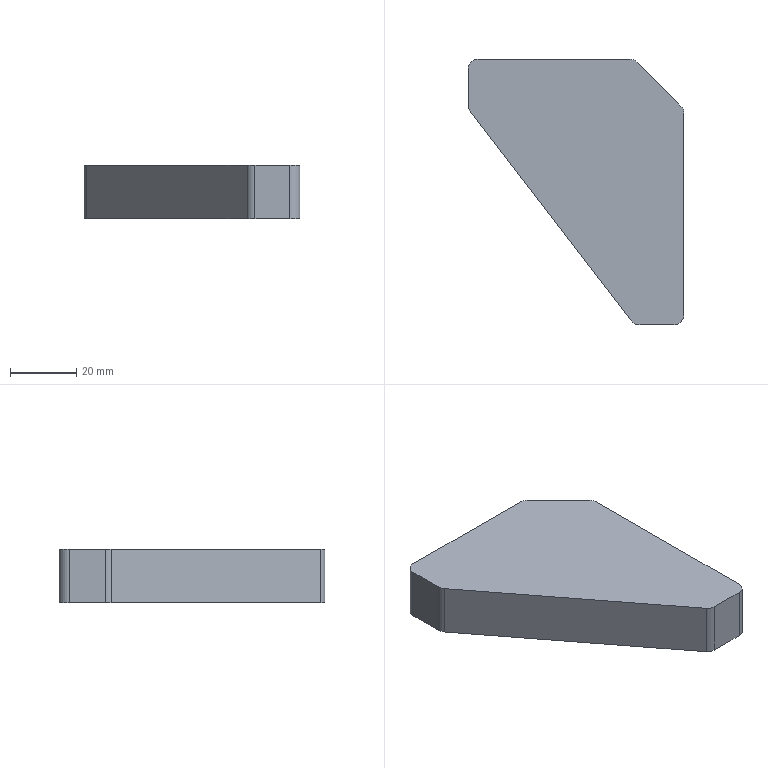Part | STEP file | SN10_008_007-03_REFORCO | 1 solid | 14 faces | box 65 x 80 x 16 mm | volume 55325 mm3 | plane 8 | cylinder 6 | commonest cylinder face diameters 6 x6
STEP:
#1=CARTESIAN_POINT('',(0.,0.,0.));
#2=DIRECTION('',(0.,0.,1.));
#3=DIRECTION('',(1.,0.,0.));
#4=AXIS2_PLACEMENT_3D('',#1,#2,#3);
#5=CARTESIAN_POINT('',(243.629,237.,420.27));
#6=VERTEX_POINT('',#5);
#7=CARTESIAN_POINT('',(246.629,240.,420.27));
#8=VERTEX_POINT('',#7);
#9=CARTESIAN_POINT('',(246.629,237.,420.27));
#10=DIRECTION('',(0.,0.,-1.));
#11=DIRECTION('',(1.,0.,0.));
#12=AXIS2_PLACEMENT_3D('',#9,#10,#11);
#13=CIRCLE('',#12,3.);
#14=CARTESIAN_POINT('',(246.629,237.,428.27));
#15=DIRECTION('',(0.,0.,-1.));
#16=DIRECTION('',(-1.,0.,0.));
#17=AXIS2_PLACEMENT_3D('',#14,#15,#16);
#18=CYLINDRICAL_SURFACE('',#17,3.);
#19=CARTESIAN_POINT('',(-3.142,8.));
#20=DIRECTION('',(1.,0.));
#21=VECTOR('',#20,1.);
#22=LINE('',#19,#21);
#23=(GEOMETRIC_REPRESENTATION_CONTEXT(2)PARAMETRIC_REPRESENTATION_CONTEXT()REPRESENTATION_CONTEXT('',''));
#24=DEFINITIONAL_REPRESENTATION('',(#22),#23);
#25=PCURVE('',#18,#24);
#26=CARTESIAN_POINT('',(0.,0.,420.27));
#27=DIRECTION('',(0.,0.,-1.));
#28=DIRECTION('',(-1.,0.,0.));
#29=AXIS2_PLACEMENT_3D('',#26,#27,#28);
#30=PLANE('',#29);
#31=CARTESIAN_POINT('',(-246.629,237.));
#32=DIRECTION('',(-1.,0.));
#33=AXIS2_PLACEMENT_2D('',#31,#32);
#34=CIRCLE('',#33,3.);
#35=(GEOMETRIC_REPRESENTATION_CONTEXT(2)PARAMETRIC_REPRESENTATION_CONTEXT()REPRESENTATION_CONTEXT('',''));
#36=DEFINITIONAL_REPRESENTATION('',(#34),#35);
#37=PCURVE('',#30,#36);
#38=SURFACE_CURVE('',#13,(#25,#37),.PCURVE_S1.);
#39=EDGE_CURVE('',#6,#8,#38,.T.);
#40=ORIENTED_EDGE('',*,*,#39,.F.);
#41=CARTESIAN_POINT('',(243.629,237.,436.27));
#42=VERTEX_POINT('',#41);
#43=CARTESIAN_POINT('',(243.629,237.,436.27));
#44=DIRECTION('',(0.,0.,-1.));
#45=VECTOR('',#44,1.);
#46=LINE('',#43,#45);
#47=CARTESIAN_POINT('',(0.,-8.));
#48=DIRECTION('',(0.,1.));
#49=VECTOR('',#48,1.);
#50=LINE('',#47,#49);
#51=(GEOMETRIC_REPRESENTATION_CONTEXT(2)PARAMETRIC_REPRESENTATION_CONTEXT()REPRESENTATION_CONTEXT('',''));
#52=DEFINITIONAL_REPRESENTATION('',(#50),#51);
#53=PCURVE('',#18,#52);
#54=CARTESIAN_POINT('',(243.629,225.,436.27));
#55=DIRECTION('',(-1.,0.,0.));
#56=DIRECTION('',(0.,0.,1.));
#57=AXIS2_PLACEMENT_3D('',#54,#55,#56);
#58=PLANE('',#57);
#59=CARTESIAN_POINT('',(0.,12.));
#60=DIRECTION('',(-1.,0.));
#61=VECTOR('',#60,1.);
#62=LINE('',#59,#61);
#63=(GEOMETRIC_REPRESENTATION_CONTEXT(2)PARAMETRIC_REPRESENTATION_CONTEXT()REPRESENTATION_CONTEXT('',''));
#64=DEFINITIONAL_REPRESENTATION('',(#62),#63);
#65=PCURVE('',#58,#64);
#66=SURFACE_CURVE('',#46,(#53,#65),.PCURVE_S1.);
#67=EDGE_CURVE('',#42,#6,#66,.T.);
#68=ORIENTED_EDGE('',*,*,#67,.F.);
#69=CARTESIAN_POINT('',(246.629,240.,436.27));
#70=VERTEX_POINT('',#69);
#71=CARTESIAN_POINT('',(246.629,237.,436.27));
#72=DIRECTION('',(0.,0.,-1.));
#73=DIRECTION('',(1.,0.,0.));
#74=AXIS2_PLACEMENT_3D('',#71,#72,#73);
#75=CIRCLE('',#74,3.);
#76=CARTESIAN_POINT('',(-3.142,-8.));
#77=DIRECTION('',(1.,0.));
#78=VECTOR('',#77,1.);
#79=LINE('',#76,#78);
#80=(GEOMETRIC_REPRESENTATION_CONTEXT(2)PARAMETRIC_REPRESENTATION_CONTEXT()REPRESENTATION_CONTEXT('',''));
#81=DEFINITIONAL_REPRESENTATION('',(#79),#80);
#82=PCURVE('',#18,#81);
#83=CARTESIAN_POINT('',(0.,0.,436.27));
#84=DIRECTION('',(0.,0.,-1.));
#85=DIRECTION('',(-1.,0.,0.));
#86=AXIS2_PLACEMENT_3D('',#83,#84,#85);
#87=PLANE('',#86);
#88=CARTESIAN_POINT('',(-246.629,237.));
#89=DIRECTION('',(-1.,0.));
#90=AXIS2_PLACEMENT_2D('',#88,#89);
#91=CIRCLE('',#90,3.);
#92=(GEOMETRIC_REPRESENTATION_CONTEXT(2)PARAMETRIC_REPRESENTATION_CONTEXT()REPRESENTATION_CONTEXT('',''));
#93=DEFINITIONAL_REPRESENTATION('',(#91),#92);
#94=PCURVE('',#87,#93);
#95=SURFACE_CURVE('',#75,(#82,#94),.PCURVE_S1.);
#96=EDGE_CURVE('',#42,#70,#95,.T.);
#97=ORIENTED_EDGE('',*,*,#96,.T.);
#98=CARTESIAN_POINT('',(246.629,240.,436.27));
#99=DIRECTION('',(0.,0.,-1.));
#100=VECTOR('',#99,1.);
#101=LINE('',#98,#100);
#102=CARTESIAN_POINT('',(1.571,-8.));
#103=DIRECTION('',(0.,1.));
#104=VECTOR('',#103,1.);
#105=LINE('',#102,#104);
#106=(GEOMETRIC_REPRESENTATION_CONTEXT(2)PARAMETRIC_REPRESENTATION_CONTEXT()REPRESENTATION_CONTEXT('',''));
#107=DEFINITIONAL_REPRESENTATION('',(#105),#106);
#108=PCURVE('',#18,#107);
#109=CARTESIAN_POINT('',(243.629,240.,436.27));
#110=DIRECTION('',(0.,1.,0.));
#111=DIRECTION('',(0.,0.,1.));
#112=AXIS2_PLACEMENT_3D('',#109,#110,#111);
#113=PLANE('',#112);
#114=CARTESIAN_POINT('',(0.,3.));
#115=DIRECTION('',(-1.,0.));
#116=VECTOR('',#115,1.);
#117=LINE('',#114,#116);
#118=(GEOMETRIC_REPRESENTATION_CONTEXT(2)PARAMETRIC_REPRESENTATION_CONTEXT()REPRESENTATION_CONTEXT('',''));
#119=DEFINITIONAL_REPRESENTATION('',(#117),#118);
#120=PCURVE('',#113,#119);
#121=SURFACE_CURVE('',#101,(#108,#120),.PCURVE_S1.);
#122=EDGE_CURVE('',#70,#8,#121,.T.);
#123=ORIENTED_EDGE('',*,*,#122,.T.);
#124=EDGE_LOOP('',(#40,#68,#97,#123));
#125=FACE_BOUND('',#124,.T.);
#126=ADVANCED_FACE('',(#125),#18,.T.);
#127=CARTESIAN_POINT('',(243.629,226.02,436.27));
#128=VERTEX_POINT('',#127);
#129=CARTESIAN_POINT('',(243.629,226.02,436.27));
#130=DIRECTION('',(0.,1.,0.));
#131=VECTOR('',#130,1.);
#132=LINE('',#129,#131);
#133=CARTESIAN_POINT('',(0.,1.02));
#134=DIRECTION('',(0.,1.));
#135=VECTOR('',#134,1.);
#136=LINE('',#133,#135);
#137=(GEOMETRIC_REPRESENTATION_CONTEXT(2)PARAMETRIC_REPRESENTATION_CONTEXT()REPRESENTATION_CONTEXT('',''));
#138=DEFINITIONAL_REPRESENTATION('',(#136),#137);
#139=PCURVE('',#58,#138);
#140=CARTESIAN_POINT('',(-243.629,226.02));
#141=DIRECTION('',(0.,1.));
#142=VECTOR('',#141,1.);
#143=LINE('',#140,#142);
#144=(GEOMETRIC_REPRESENTATION_CONTEXT(2)PARAMETRIC_REPRESENTATION_CONTEXT()REPRESENTATION_CONTEXT('',''));
#145=DEFINITIONAL_REPRESENTATION('',(#143),#144);
#146=PCURVE('',#87,#145);
#147=SURFACE_CURVE('',#132,(#139,#146),.PCURVE_S1.);
#148=EDGE_CURVE('',#128,#42,#147,.T.);
#149=ORIENTED_EDGE('',*,*,#148,.T.);
#150=ORIENTED_EDGE('',*,*,#67,.T.);
#151=CARTESIAN_POINT('',(243.629,226.02,420.27));
#152=VERTEX_POINT('',#151);
#153=CARTESIAN_POINT('',(243.629,226.02,420.27));
#154=DIRECTION('',(0.,1.,0.));
#155=VECTOR('',#154,1.);
#156=LINE('',#153,#155);
#157=CARTESIAN_POINT('',(-16.,1.02));
#158=DIRECTION('',(0.,1.));
#159=VECTOR('',#158,1.);
#160=LINE('',#157,#159);
#161=(GEOMETRIC_REPRESENTATION_CONTEXT(2)PARAMETRIC_REPRESENTATION_CONTEXT()REPRESENTATION_CONTEXT('',''));
#162=DEFINITIONAL_REPRESENTATION('',(#160),#161);
#163=PCURVE('',#58,#162);
#164=CARTESIAN_POINT('',(-243.629,226.02));
#165=DIRECTION('',(0.,1.));
#166=VECTOR('',#165,1.);
#167=LINE('',#164,#166);
#168=(GEOMETRIC_REPRESENTATION_CONTEXT(2)PARAMETRIC_REPRESENTATION_CONTEXT()REPRESENTATION_CONTEXT('',''));
#169=DEFINITIONAL_REPRESENTATION('',(#167),#168);
#170=PCURVE('',#30,#169);
#171=SURFACE_CURVE('',#156,(#163,#170),.PCURVE_S1.);
#172=EDGE_CURVE('',#152,#6,#171,.T.);
#173=ORIENTED_EDGE('',*,*,#172,.F.);
#174=CARTESIAN_POINT('',(243.629,226.02,436.27));
#175=DIRECTION('',(0.,0.,-1.));
#176=VECTOR('',#175,1.);
#177=LINE('',#174,#176);
#178=CARTESIAN_POINT('',(0.,1.02));
#179=DIRECTION('',(-1.,0.));
#180=VECTOR('',#179,1.);
#181=LINE('',#178,#180);
#182=(GEOMETRIC_REPRESENTATION_CONTEXT(2)PARAMETRIC_REPRESENTATION_CONTEXT()REPRESENTATION_CONTEXT('',''));
#183=DEFINITIONAL_REPRESENTATION('',(#181),#182);
#184=PCURVE('',#58,#183);
#185=CARTESIAN_POINT('',(246.629,226.02,428.27));
#186=DIRECTION('',(0.,0.,-1.));
#187=DIRECTION('',(-0.7926,-0.6097,0.));
#188=AXIS2_PLACEMENT_3D('',#185,#186,#187);
#189=CYLINDRICAL_SURFACE('',#188,3.);
#190=CARTESIAN_POINT('',(0.6557,-8.));
#191=DIRECTION('',(0.,1.));
#192=VECTOR('',#191,1.);
#193=LINE('',#190,#192);
#194=(GEOMETRIC_REPRESENTATION_CONTEXT(2)PARAMETRIC_REPRESENTATION_CONTEXT()REPRESENTATION_CONTEXT('',''));
#195=DEFINITIONAL_REPRESENTATION('',(#193),#194);
#196=PCURVE('',#189,#195);
#197=SURFACE_CURVE('',#177,(#184,#196),.PCURVE_S1.);
#198=EDGE_CURVE('',#128,#152,#197,.T.);
#199=ORIENTED_EDGE('',*,*,#198,.F.);
#200=EDGE_LOOP('',(#149,#150,#173,#199));
#201=FACE_BOUND('',#200,.T.);
#202=ADVANCED_FACE('',(#201),#58,.T.);
#203=CARTESIAN_POINT('',(244.251,224.191,420.27));
#204=VERTEX_POINT('',#203);
#205=CARTESIAN_POINT('',(246.629,226.02,420.27));
#206=DIRECTION('',(0.,0.,-1.));
#207=DIRECTION('',(1.,0.,0.));
#208=AXIS2_PLACEMENT_3D('',#205,#206,#207);
#209=CIRCLE('',#208,3.);
#210=CARTESIAN_POINT('',(-2.486,8.));
#211=DIRECTION('',(1.,0.));
#212=VECTOR('',#211,1.);
#213=LINE('',#210,#212);
#214=(GEOMETRIC_REPRESENTATION_CONTEXT(2)PARAMETRIC_REPRESENTATION_CONTEXT()REPRESENTATION_CONTEXT('',''));
#215=DEFINITIONAL_REPRESENTATION('',(#213),#214);
#216=PCURVE('',#189,#215);
#217=CARTESIAN_POINT('',(-246.629,226.02));
#218=DIRECTION('',(-1.,0.));
#219=AXIS2_PLACEMENT_2D('',#217,#218);
#220=CIRCLE('',#219,3.);
#221=(GEOMETRIC_REPRESENTATION_CONTEXT(2)PARAMETRIC_REPRESENTATION_CONTEXT()REPRESENTATION_CONTEXT('',''));
#222=DEFINITIONAL_REPRESENTATION('',(#220),#221);
#223=PCURVE('',#30,#222);
#224=SURFACE_CURVE('',#209,(#216,#223),.PCURVE_S1.);
#225=EDGE_CURVE('',#204,#152,#224,.T.);
#226=ORIENTED_EDGE('',*,*,#225,.F.);
#227=CARTESIAN_POINT('',(244.251,224.191,436.27));
#228=VERTEX_POINT('',#227);
#229=CARTESIAN_POINT('',(244.251,224.191,436.27));
#230=DIRECTION('',(0.,0.,-1.));
#231=VECTOR('',#230,1.);
#232=LINE('',#229,#231);
#233=CARTESIAN_POINT('',(0.,-8.));
#234=DIRECTION('',(0.,1.));
#235=VECTOR('',#234,1.);
#236=LINE('',#233,#235);
#237=(GEOMETRIC_REPRESENTATION_CONTEXT(2)PARAMETRIC_REPRESENTATION_CONTEXT()REPRESENTATION_CONTEXT('',''));
#238=DEFINITIONAL_REPRESENTATION('',(#236),#237);
#239=PCURVE('',#189,#238);
#240=CARTESIAN_POINT('',(293.629,160.,436.27));
#241=DIRECTION('',(-0.7926,-0.6097,0.));
#242=DIRECTION('',(0.,0.,1.));
#243=AXIS2_PLACEMENT_3D('',#240,#241,#242);
#244=PLANE('',#243);
#245=CARTESIAN_POINT('',(0.,80.986));
#246=DIRECTION('',(-1.,0.));
#247=VECTOR('',#246,1.);
#248=LINE('',#245,#247);
#249=(GEOMETRIC_REPRESENTATION_CONTEXT(2)PARAMETRIC_REPRESENTATION_CONTEXT()REPRESENTATION_CONTEXT('',''));
#250=DEFINITIONAL_REPRESENTATION('',(#248),#249);
#251=PCURVE('',#244,#250);
#252=SURFACE_CURVE('',#232,(#239,#251),.PCURVE_S1.);
#253=EDGE_CURVE('',#228,#204,#252,.T.);
#254=ORIENTED_EDGE('',*,*,#253,.F.);
#255=CARTESIAN_POINT('',(246.629,226.02,436.27));
#256=DIRECTION('',(0.,0.,-1.));
#257=DIRECTION('',(1.,0.,0.));
#258=AXIS2_PLACEMENT_3D('',#255,#256,#257);
#259=CIRCLE('',#258,3.);
#260=CARTESIAN_POINT('',(-2.486,-8.));
#261=DIRECTION('',(1.,0.));
#262=VECTOR('',#261,1.);
#263=LINE('',#260,#262);
#264=(GEOMETRIC_REPRESENTATION_CONTEXT(2)PARAMETRIC_REPRESENTATION_CONTEXT()REPRESENTATION_CONTEXT('',''));
#265=DEFINITIONAL_REPRESENTATION('',(#263),#264);
#266=PCURVE('',#189,#265);
#267=CARTESIAN_POINT('',(-246.629,226.02));
#268=DIRECTION('',(-1.,0.));
#269=AXIS2_PLACEMENT_2D('',#267,#268);
#270=CIRCLE('',#269,3.);
#271=(GEOMETRIC_REPRESENTATION_CONTEXT(2)PARAMETRIC_REPRESENTATION_CONTEXT()REPRESENTATION_CONTEXT('',''));
#272=DEFINITIONAL_REPRESENTATION('',(#270),#271);
#273=PCURVE('',#87,#272);
#274=SURFACE_CURVE('',#259,(#266,#273),.PCURVE_S1.);
#275=EDGE_CURVE('',#228,#128,#274,.T.);
#276=ORIENTED_EDGE('',*,*,#275,.T.);
#277=ORIENTED_EDGE('',*,*,#198,.T.);
#278=EDGE_LOOP('',(#226,#254,#276,#277));
#279=FACE_BOUND('',#278,.T.);
#280=ADVANCED_FACE('',(#279),#189,.T.);
#281=CARTESIAN_POINT('',(292.728,161.171,436.27));
#282=VERTEX_POINT('',#281);
#283=CARTESIAN_POINT('',(292.728,161.171,436.27));
#284=DIRECTION('',(-0.6097,0.7926,0.));
#285=VECTOR('',#284,1.);
#286=LINE('',#283,#285);
#287=CARTESIAN_POINT('',(0.,1.477));
#288=DIRECTION('',(0.,1.));
#289=VECTOR('',#288,1.);
#290=LINE('',#287,#289);
#291=(GEOMETRIC_REPRESENTATION_CONTEXT(2)PARAMETRIC_REPRESENTATION_CONTEXT()REPRESENTATION_CONTEXT('',''));
#292=DEFINITIONAL_REPRESENTATION('',(#290),#291);
#293=PCURVE('',#244,#292);
#294=CARTESIAN_POINT('',(-292.728,161.171));
#295=DIRECTION('',(0.6097,0.7926));
#296=VECTOR('',#295,1.);
#297=LINE('',#294,#296);
#298=(GEOMETRIC_REPRESENTATION_CONTEXT(2)PARAMETRIC_REPRESENTATION_CONTEXT()REPRESENTATION_CONTEXT('',''));
#299=DEFINITIONAL_REPRESENTATION('',(#297),#298);
#300=PCURVE('',#87,#299);
#301=SURFACE_CURVE('',#286,(#293,#300),.PCURVE_S1.);
#302=EDGE_CURVE('',#282,#228,#301,.T.);
#303=ORIENTED_EDGE('',*,*,#302,.T.);
#304=ORIENTED_EDGE('',*,*,#253,.T.);
#305=CARTESIAN_POINT('',(292.728,161.171,420.27));
#306=VERTEX_POINT('',#305);
#307=CARTESIAN_POINT('',(292.728,161.171,420.27));
#308=DIRECTION('',(-0.6097,0.7926,0.));
#309=VECTOR('',#308,1.);
#310=LINE('',#307,#309);
#311=CARTESIAN_POINT('',(-16.,1.477));
#312=DIRECTION('',(0.,1.));
#313=VECTOR('',#312,1.);
#314=LINE('',#311,#313);
#315=(GEOMETRIC_REPRESENTATION_CONTEXT(2)PARAMETRIC_REPRESENTATION_CONTEXT()REPRESENTATION_CONTEXT('',''));
#316=DEFINITIONAL_REPRESENTATION('',(#314),#315);
#317=PCURVE('',#244,#316);
#318=CARTESIAN_POINT('',(-292.728,161.171));
#319=DIRECTION('',(0.6097,0.7926));
#320=VECTOR('',#319,1.);
#321=LINE('',#318,#320);
#322=(GEOMETRIC_REPRESENTATION_CONTEXT(2)PARAMETRIC_REPRESENTATION_CONTEXT()REPRESENTATION_CONTEXT('',''));
#323=DEFINITIONAL_REPRESENTATION('',(#321),#322);
#324=PCURVE('',#30,#323);
#325=SURFACE_CURVE('',#310,(#317,#324),.PCURVE_S1.);
#326=EDGE_CURVE('',#306,#204,#325,.T.);
#327=ORIENTED_EDGE('',*,*,#326,.F.);
#328=CARTESIAN_POINT('',(292.728,161.171,436.27));
#329=DIRECTION('',(0.,0.,-1.));
#330=VECTOR('',#329,1.);
#331=LINE('',#328,#330);
#332=CARTESIAN_POINT('',(0.,1.477));
#333=DIRECTION('',(-1.,0.));
#334=VECTOR('',#333,1.);
#335=LINE('',#332,#334);
#336=(GEOMETRIC_REPRESENTATION_CONTEXT(2)PARAMETRIC_REPRESENTATION_CONTEXT()REPRESENTATION_CONTEXT('',''));
#337=DEFINITIONAL_REPRESENTATION('',(#335),#336);
#338=PCURVE('',#244,#337);
#339=CARTESIAN_POINT('',(295.106,163.,428.27));
#340=DIRECTION('',(0.,0.,-1.));
#341=DIRECTION('',(0.,-1.,0.));
#342=AXIS2_PLACEMENT_3D('',#339,#340,#341);
#343=CYLINDRICAL_SURFACE('',#342,3.);
#344=CARTESIAN_POINT('',(0.9151,-8.));
#345=DIRECTION('',(0.,1.));
#346=VECTOR('',#345,1.);
#347=LINE('',#344,#346);
#348=(GEOMETRIC_REPRESENTATION_CONTEXT(2)PARAMETRIC_REPRESENTATION_CONTEXT()REPRESENTATION_CONTEXT('',''));
#349=DEFINITIONAL_REPRESENTATION('',(#347),#348);
#350=PCURVE('',#343,#349);
#351=SURFACE_CURVE('',#331,(#338,#350),.PCURVE_S1.);
#352=EDGE_CURVE('',#282,#306,#351,.T.);
#353=ORIENTED_EDGE('',*,*,#352,.F.);
#354=EDGE_LOOP('',(#303,#304,#327,#353));
#355=FACE_BOUND('',#354,.T.);
#356=ADVANCED_FACE('',(#355),#244,.T.);
#357=CARTESIAN_POINT('',(295.106,160.,420.27));
#358=VERTEX_POINT('',#357);
#359=CARTESIAN_POINT('',(295.106,163.,420.27));
#360=DIRECTION('',(0.,0.,-1.));
#361=DIRECTION('',(1.,0.,0.));
#362=AXIS2_PLACEMENT_3D('',#359,#360,#361);
#363=CIRCLE('',#362,3.);
#364=CARTESIAN_POINT('',(-1.571,8.));
#365=DIRECTION('',(1.,0.));
#366=VECTOR('',#365,1.);
#367=LINE('',#364,#366);
#368=(GEOMETRIC_REPRESENTATION_CONTEXT(2)PARAMETRIC_REPRESENTATION_CONTEXT()REPRESENTATION_CONTEXT('',''));
#369=DEFINITIONAL_REPRESENTATION('',(#367),#368);
#370=PCURVE('',#343,#369);
#371=CARTESIAN_POINT('',(-295.106,163.));
#372=DIRECTION('',(-1.,0.));
#373=AXIS2_PLACEMENT_2D('',#371,#372);
#374=CIRCLE('',#373,3.);
#375=(GEOMETRIC_REPRESENTATION_CONTEXT(2)PARAMETRIC_REPRESENTATION_CONTEXT()REPRESENTATION_CONTEXT('',''));
#376=DEFINITIONAL_REPRESENTATION('',(#374),#375);
#377=PCURVE('',#30,#376);
#378=SURFACE_CURVE('',#363,(#370,#377),.PCURVE_S1.);
#379=EDGE_CURVE('',#358,#306,#378,.T.);
#380=ORIENTED_EDGE('',*,*,#379,.F.);
#381=CARTESIAN_POINT('',(295.106,160.,436.27));
#382=VERTEX_POINT('',#381);
#383=CARTESIAN_POINT('',(295.106,160.,436.27));
#384=DIRECTION('',(0.,0.,-1.));
#385=VECTOR('',#384,1.);
#386=LINE('',#383,#385);
#387=CARTESIAN_POINT('',(0.,-8.));
#388=DIRECTION('',(0.,1.));
#389=VECTOR('',#388,1.);
#390=LINE('',#387,#389);
#391=(GEOMETRIC_REPRESENTATION_CONTEXT(2)PARAMETRIC_REPRESENTATION_CONTEXT()REPRESENTATION_CONTEXT('',''));
#392=DEFINITIONAL_REPRESENTATION('',(#390),#391);
#393=PCURVE('',#343,#392);
#394=CARTESIAN_POINT('',(308.629,160.,436.27));
#395=DIRECTION('',(0.,-1.,0.));
#396=DIRECTION('',(0.,0.,-1.));
#397=AXIS2_PLACEMENT_3D('',#394,#395,#396);
#398=PLANE('',#397);
#399=CARTESIAN_POINT('',(0.,-13.523));
#400=DIRECTION('',(1.,0.));
#401=VECTOR('',#400,1.);
#402=LINE('',#399,#401);
#403=(GEOMETRIC_REPRESENTATION_CONTEXT(2)PARAMETRIC_REPRESENTATION_CONTEXT()REPRESENTATION_CONTEXT('',''));
#404=DEFINITIONAL_REPRESENTATION('',(#402),#403);
#405=PCURVE('',#398,#404);
#406=SURFACE_CURVE('',#386,(#393,#405),.PCURVE_S1.);
#407=EDGE_CURVE('',#382,#358,#406,.T.);
#408=ORIENTED_EDGE('',*,*,#407,.F.);
#409=CARTESIAN_POINT('',(295.106,163.,436.27));
#410=DIRECTION('',(0.,0.,-1.));
#411=DIRECTION('',(1.,0.,0.));
#412=AXIS2_PLACEMENT_3D('',#409,#410,#411);
#413=CIRCLE('',#412,3.);
#414=CARTESIAN_POINT('',(-1.571,-8.));
#415=DIRECTION('',(1.,0.));
#416=VECTOR('',#415,1.);
#417=LINE('',#414,#416);
#418=(GEOMETRIC_REPRESENTATION_CONTEXT(2)PARAMETRIC_REPRESENTATION_CONTEXT()REPRESENTATION_CONTEXT('',''));
#419=DEFINITIONAL_REPRESENTATION('',(#417),#418);
#420=PCURVE('',#343,#419);
#421=CARTESIAN_POINT('',(-295.106,163.));
#422=DIRECTION('',(-1.,0.));
#423=AXIS2_PLACEMENT_2D('',#421,#422);
#424=CIRCLE('',#423,3.);
#425=(GEOMETRIC_REPRESENTATION_CONTEXT(2)PARAMETRIC_REPRESENTATION_CONTEXT()REPRESENTATION_CONTEXT('',''));
#426=DEFINITIONAL_REPRESENTATION('',(#424),#425);
#427=PCURVE('',#87,#426);
#428=SURFACE_CURVE('',#413,(#420,#427),.PCURVE_S1.);
#429=EDGE_CURVE('',#382,#282,#428,.T.);
#430=ORIENTED_EDGE('',*,*,#429,.T.);
#431=ORIENTED_EDGE('',*,*,#352,.T.);
#432=EDGE_LOOP('',(#380,#408,#430,#431));
#433=FACE_BOUND('',#432,.T.);
#434=ADVANCED_FACE('',(#433),#343,.T.);
#435=CARTESIAN_POINT('',(305.629,160.,436.27));
#436=VERTEX_POINT('',#435);
#437=CARTESIAN_POINT('',(305.629,160.,436.27));
#438=DIRECTION('',(-1.,0.,0.));
#439=VECTOR('',#438,1.);
#440=LINE('',#437,#439);
#441=CARTESIAN_POINT('',(0.,-3.));
#442=DIRECTION('',(0.,-1.));
#443=VECTOR('',#442,1.);
#444=LINE('',#441,#443);
#445=(GEOMETRIC_REPRESENTATION_CONTEXT(2)PARAMETRIC_REPRESENTATION_CONTEXT()REPRESENTATION_CONTEXT('',''));
#446=DEFINITIONAL_REPRESENTATION('',(#444),#445);
#447=PCURVE('',#398,#446);
#448=CARTESIAN_POINT('',(-305.629,160.));
#449=DIRECTION('',(1.,0.));
#450=VECTOR('',#449,1.);
#451=LINE('',#448,#450);
#452=(GEOMETRIC_REPRESENTATION_CONTEXT(2)PARAMETRIC_REPRESENTATION_CONTEXT()REPRESENTATION_CONTEXT('',''));
#453=DEFINITIONAL_REPRESENTATION('',(#451),#452);
#454=PCURVE('',#87,#453);
#455=SURFACE_CURVE('',#440,(#447,#454),.PCURVE_S1.);
#456=EDGE_CURVE('',#436,#382,#455,.T.);
#457=ORIENTED_EDGE('',*,*,#456,.T.);
#458=ORIENTED_EDGE('',*,*,#407,.T.);
#459=CARTESIAN_POINT('',(305.629,160.,420.27));
#460=VERTEX_POINT('',#459);
#461=CARTESIAN_POINT('',(305.629,160.,420.27));
#462=DIRECTION('',(-1.,0.,0.));
#463=VECTOR('',#462,1.);
#464=LINE('',#461,#463);
#465=CARTESIAN_POINT('',(16.,-3.));
#466=DIRECTION('',(0.,-1.));
#467=VECTOR('',#466,1.);
#468=LINE('',#465,#467);
#469=(GEOMETRIC_REPRESENTATION_CONTEXT(2)PARAMETRIC_REPRESENTATION_CONTEXT()REPRESENTATION_CONTEXT('',''));
#470=DEFINITIONAL_REPRESENTATION('',(#468),#469);
#471=PCURVE('',#398,#470);
#472=CARTESIAN_POINT('',(-305.629,160.));
#473=DIRECTION('',(1.,0.));
#474=VECTOR('',#473,1.);
#475=LINE('',#472,#474);
#476=(GEOMETRIC_REPRESENTATION_CONTEXT(2)PARAMETRIC_REPRESENTATION_CONTEXT()REPRESENTATION_CONTEXT('',''));
#477=DEFINITIONAL_REPRESENTATION('',(#475),#476);
#478=PCURVE('',#30,#477);
#479=SURFACE_CURVE('',#464,(#471,#478),.PCURVE_S1.);
#480=EDGE_CURVE('',#460,#358,#479,.T.);
#481=ORIENTED_EDGE('',*,*,#480,.F.);
#482=CARTESIAN_POINT('',(305.629,160.,436.27));
#483=DIRECTION('',(0.,0.,-1.));
#484=VECTOR('',#483,1.);
#485=LINE('',#482,#484);
#486=CARTESIAN_POINT('',(0.,-3.));
#487=DIRECTION('',(1.,0.));
#488=VECTOR('',#487,1.);
#489=LINE('',#486,#488);
#490=(GEOMETRIC_REPRESENTATION_CONTEXT(2)PARAMETRIC_REPRESENTATION_CONTEXT()REPRESENTATION_CONTEXT('',''));
#491=DEFINITIONAL_REPRESENTATION('',(#489),#490);
#492=PCURVE('',#398,#491);
#493=CARTESIAN_POINT('',(305.629,163.,428.27));
#494=DIRECTION('',(0.,0.,-1.));
#495=DIRECTION('',(1.,0.,0.));
#496=AXIS2_PLACEMENT_3D('',#493,#494,#495);
#497=CYLINDRICAL_SURFACE('',#496,3.);
#498=CARTESIAN_POINT('',(1.571,-8.));
#499=DIRECTION('',(0.,1.));
#500=VECTOR('',#499,1.);
#501=LINE('',#498,#500);
#502=(GEOMETRIC_REPRESENTATION_CONTEXT(2)PARAMETRIC_REPRESENTATION_CONTEXT()REPRESENTATION_CONTEXT('',''));
#503=DEFINITIONAL_REPRESENTATION('',(#501),#502);
#504=PCURVE('',#497,#503);
#505=SURFACE_CURVE('',#485,(#492,#504),.PCURVE_S1.);
#506=EDGE_CURVE('',#436,#460,#505,.T.);
#507=ORIENTED_EDGE('',*,*,#506,.F.);
#508=EDGE_LOOP('',(#457,#458,#481,#507));
#509=FACE_BOUND('',#508,.T.);
#510=ADVANCED_FACE('',(#509),#398,.T.);
#511=CARTESIAN_POINT('',(308.629,163.,420.27));
#512=VERTEX_POINT('',#511);
#513=CARTESIAN_POINT('',(305.629,163.,420.27));
#514=DIRECTION('',(0.,0.,-1.));
#515=DIRECTION('',(1.,0.,0.));
#516=AXIS2_PLACEMENT_3D('',#513,#514,#515);
#517=CIRCLE('',#516,3.);
#518=CARTESIAN_POINT('',(0.,8.));
#519=DIRECTION('',(1.,0.));
#520=VECTOR('',#519,1.);
#521=LINE('',#518,#520);
#522=(GEOMETRIC_REPRESENTATION_CONTEXT(2)PARAMETRIC_REPRESENTATION_CONTEXT()REPRESENTATION_CONTEXT('',''));
#523=DEFINITIONAL_REPRESENTATION('',(#521),#522);
#524=PCURVE('',#497,#523);
#525=CARTESIAN_POINT('',(-305.629,163.));
#526=DIRECTION('',(-1.,0.));
#527=AXIS2_PLACEMENT_2D('',#525,#526);
#528=CIRCLE('',#527,3.);
#529=(GEOMETRIC_REPRESENTATION_CONTEXT(2)PARAMETRIC_REPRESENTATION_CONTEXT()REPRESENTATION_CONTEXT('',''));
#530=DEFINITIONAL_REPRESENTATION('',(#528),#529);
#531=PCURVE('',#30,#530);
#532=SURFACE_CURVE('',#517,(#524,#531),.PCURVE_S1.);
#533=EDGE_CURVE('',#512,#460,#532,.T.);
#534=ORIENTED_EDGE('',*,*,#533,.F.);
#535=CARTESIAN_POINT('',(308.629,163.,436.27));
#536=VERTEX_POINT('',#535);
#537=CARTESIAN_POINT('',(308.629,163.,436.27));
#538=DIRECTION('',(0.,0.,-1.));
#539=VECTOR('',#538,1.);
#540=LINE('',#537,#539);
#541=CARTESIAN_POINT('',(0.,-8.));
#542=DIRECTION('',(0.,1.));
#543=VECTOR('',#542,1.);
#544=LINE('',#541,#543);
#545=(GEOMETRIC_REPRESENTATION_CONTEXT(2)PARAMETRIC_REPRESENTATION_CONTEXT()REPRESENTATION_CONTEXT('',''));
#546=DEFINITIONAL_REPRESENTATION('',(#544),#545);
#547=PCURVE('',#497,#546);
#548=CARTESIAN_POINT('',(308.629,225.,436.27));
#549=DIRECTION('',(1.,0.,0.));
#550=DIRECTION('',(0.,0.,-1.));
#551=AXIS2_PLACEMENT_3D('',#548,#549,#550);
#552=PLANE('',#551);
#553=CARTESIAN_POINT('',(0.,-62.));
#554=DIRECTION('',(1.,0.));
#555=VECTOR('',#554,1.);
#556=LINE('',#553,#555);
#557=(GEOMETRIC_REPRESENTATION_CONTEXT(2)PARAMETRIC_REPRESENTATION_CONTEXT()REPRESENTATION_CONTEXT('',''));
#558=DEFINITIONAL_REPRESENTATION('',(#556),#557);
#559=PCURVE('',#552,#558);
#560=SURFACE_CURVE('',#540,(#547,#559),.PCURVE_S1.);
#561=EDGE_CURVE('',#536,#512,#560,.T.);
#562=ORIENTED_EDGE('',*,*,#561,.F.);
#563=CARTESIAN_POINT('',(305.629,163.,436.27));
#564=DIRECTION('',(0.,0.,-1.));
#565=DIRECTION('',(1.,0.,0.));
#566=AXIS2_PLACEMENT_3D('',#563,#564,#565);
#567=CIRCLE('',#566,3.);
#568=CARTESIAN_POINT('',(0.,-8.));
#569=DIRECTION('',(1.,0.));
#570=VECTOR('',#569,1.);
#571=LINE('',#568,#570);
#572=(GEOMETRIC_REPRESENTATION_CONTEXT(2)PARAMETRIC_REPRESENTATION_CONTEXT()REPRESENTATION_CONTEXT('',''));
#573=DEFINITIONAL_REPRESENTATION('',(#571),#572);
#574=PCURVE('',#497,#573);
#575=CARTESIAN_POINT('',(-305.629,163.));
#576=DIRECTION('',(-1.,0.));
#577=AXIS2_PLACEMENT_2D('',#575,#576);
#578=CIRCLE('',#577,3.);
#579=(GEOMETRIC_REPRESENTATION_CONTEXT(2)PARAMETRIC_REPRESENTATION_CONTEXT()REPRESENTATION_CONTEXT('',''));
#580=DEFINITIONAL_REPRESENTATION('',(#578),#579);
#581=PCURVE('',#87,#580);
#582=SURFACE_CURVE('',#567,(#574,#581),.PCURVE_S1.);
#583=EDGE_CURVE('',#536,#436,#582,.T.);
#584=ORIENTED_EDGE('',*,*,#583,.T.);
#585=ORIENTED_EDGE('',*,*,#506,.T.);
#586=EDGE_LOOP('',(#534,#562,#584,#585));
#587=FACE_BOUND('',#586,.T.);
#588=ADVANCED_FACE('',(#587),#497,.T.);
#589=CARTESIAN_POINT('',(308.629,223.757,436.27));
#590=VERTEX_POINT('',#589);
#591=CARTESIAN_POINT('',(308.629,223.757,436.27));
#592=DIRECTION('',(0.,-1.,0.));
#593=VECTOR('',#592,1.);
#594=LINE('',#591,#593);
#595=CARTESIAN_POINT('',(0.,-1.243));
#596=DIRECTION('',(0.,-1.));
#597=VECTOR('',#596,1.);
#598=LINE('',#595,#597);
#599=(GEOMETRIC_REPRESENTATION_CONTEXT(2)PARAMETRIC_REPRESENTATION_CONTEXT()REPRESENTATION_CONTEXT('',''));
#600=DEFINITIONAL_REPRESENTATION('',(#598),#599);
#601=PCURVE('',#552,#600);
#602=CARTESIAN_POINT('',(-308.629,223.757));
#603=DIRECTION('',(0.,-1.));
#604=VECTOR('',#603,1.);
#605=LINE('',#602,#604);
#606=(GEOMETRIC_REPRESENTATION_CONTEXT(2)PARAMETRIC_REPRESENTATION_CONTEXT()REPRESENTATION_CONTEXT('',''));
#607=DEFINITIONAL_REPRESENTATION('',(#605),#606);
#608=PCURVE('',#87,#607);
#609=SURFACE_CURVE('',#594,(#601,#608),.PCURVE_S1.);
#610=EDGE_CURVE('',#590,#536,#609,.T.);
#611=ORIENTED_EDGE('',*,*,#610,.T.);
#612=ORIENTED_EDGE('',*,*,#561,.T.);
#613=CARTESIAN_POINT('',(308.629,223.757,420.27));
#614=VERTEX_POINT('',#613);
#615=CARTESIAN_POINT('',(308.629,223.757,420.27));
#616=DIRECTION('',(0.,-1.,0.));
#617=VECTOR('',#616,1.);
#618=LINE('',#615,#617);
#619=CARTESIAN_POINT('',(16.,-1.243));
#620=DIRECTION('',(0.,-1.));
#621=VECTOR('',#620,1.);
#622=LINE('',#619,#621);
#623=(GEOMETRIC_REPRESENTATION_CONTEXT(2)PARAMETRIC_REPRESENTATION_CONTEXT()REPRESENTATION_CONTEXT('',''));
#624=DEFINITIONAL_REPRESENTATION('',(#622),#623);
#625=PCURVE('',#552,#624);
#626=CARTESIAN_POINT('',(-308.629,223.757));
#627=DIRECTION('',(0.,-1.));
#628=VECTOR('',#627,1.);
#629=LINE('',#626,#628);
#630=(GEOMETRIC_REPRESENTATION_CONTEXT(2)PARAMETRIC_REPRESENTATION_CONTEXT()REPRESENTATION_CONTEXT('',''));
#631=DEFINITIONAL_REPRESENTATION('',(#629),#630);
#632=PCURVE('',#30,#631);
#633=SURFACE_CURVE('',#618,(#625,#632),.PCURVE_S1.);
#634=EDGE_CURVE('',#614,#512,#633,.T.);
#635=ORIENTED_EDGE('',*,*,#634,.F.);
#636=CARTESIAN_POINT('',(308.629,223.757,436.27));
#637=DIRECTION('',(0.,0.,-1.));
#638=VECTOR('',#637,1.);
#639=LINE('',#636,#638);
#640=CARTESIAN_POINT('',(0.,-1.243));
#641=DIRECTION('',(1.,0.));
#642=VECTOR('',#641,1.);
#643=LINE('',#640,#642);
#644=(GEOMETRIC_REPRESENTATION_CONTEXT(2)PARAMETRIC_REPRESENTATION_CONTEXT()REPRESENTATION_CONTEXT('',''));
#645=DEFINITIONAL_REPRESENTATION('',(#643),#644);
#646=PCURVE('',#552,#645);
#647=CARTESIAN_POINT('',(305.629,223.757,428.27));
#648=DIRECTION('',(0.,0.,-1.));
#649=DIRECTION('',(0.7071,0.7071,0.));
#650=AXIS2_PLACEMENT_3D('',#647,#648,#649);
#651=CYLINDRICAL_SURFACE('',#650,3.);
#652=CARTESIAN_POINT('',(0.7854,-8.));
#653=DIRECTION('',(0.,1.));
#654=VECTOR('',#653,1.);
#655=LINE('',#652,#654);
#656=(GEOMETRIC_REPRESENTATION_CONTEXT(2)PARAMETRIC_REPRESENTATION_CONTEXT()REPRESENTATION_CONTEXT('',''));
#657=DEFINITIONAL_REPRESENTATION('',(#655),#656);
#658=PCURVE('',#651,#657);
#659=SURFACE_CURVE('',#639,(#646,#658),.PCURVE_S1.);
#660=EDGE_CURVE('',#590,#614,#659,.T.);
#661=ORIENTED_EDGE('',*,*,#660,.F.);
#662=EDGE_LOOP('',(#611,#612,#635,#661));
#663=FACE_BOUND('',#662,.T.);
#664=ADVANCED_FACE('',(#663),#552,.T.);
#665=CARTESIAN_POINT('',(307.75,225.879,420.27));
#666=VERTEX_POINT('',#665);
#667=CARTESIAN_POINT('',(305.629,223.757,420.27));
#668=DIRECTION('',(0.,0.,-1.));
#669=DIRECTION('',(1.,0.,0.));
#670=AXIS2_PLACEMENT_3D('',#667,#668,#669);
#671=CIRCLE('',#670,3.);
#672=CARTESIAN_POINT('',(-5.498,8.));
#673=DIRECTION('',(1.,0.));
#674=VECTOR('',#673,1.);
#675=LINE('',#672,#674);
#676=(GEOMETRIC_REPRESENTATION_CONTEXT(2)PARAMETRIC_REPRESENTATION_CONTEXT()REPRESENTATION_CONTEXT('',''));
#677=DEFINITIONAL_REPRESENTATION('',(#675),#676);
#678=PCURVE('',#651,#677);
#679=CARTESIAN_POINT('',(-305.629,223.757));
#680=DIRECTION('',(-1.,0.));
#681=AXIS2_PLACEMENT_2D('',#679,#680);
#682=CIRCLE('',#681,3.);
#683=(GEOMETRIC_REPRESENTATION_CONTEXT(2)PARAMETRIC_REPRESENTATION_CONTEXT()REPRESENTATION_CONTEXT('',''));
#684=DEFINITIONAL_REPRESENTATION('',(#682),#683);
#685=PCURVE('',#30,#684);
#686=SURFACE_CURVE('',#671,(#678,#685),.PCURVE_S1.);
#687=EDGE_CURVE('',#666,#614,#686,.T.);
#688=ORIENTED_EDGE('',*,*,#687,.F.);
#689=CARTESIAN_POINT('',(307.75,225.879,436.27));
#690=VERTEX_POINT('',#689);
#691=CARTESIAN_POINT('',(307.75,225.879,436.27));
#692=DIRECTION('',(0.,0.,-1.));
#693=VECTOR('',#692,1.);
#694=LINE('',#691,#693);
#695=CARTESIAN_POINT('',(0.,-8.));
#696=DIRECTION('',(0.,1.));
#697=VECTOR('',#696,1.);
#698=LINE('',#695,#697);
#699=(GEOMETRIC_REPRESENTATION_CONTEXT(2)PARAMETRIC_REPRESENTATION_CONTEXT()REPRESENTATION_CONTEXT('',''));
#700=DEFINITIONAL_REPRESENTATION('',(#698),#699);
#701=PCURVE('',#651,#700);
#702=CARTESIAN_POINT('',(293.629,240.,436.27));
#703=DIRECTION('',(0.7071,0.7071,0.));
#704=DIRECTION('',(0.,0.,-1.));
#705=AXIS2_PLACEMENT_3D('',#702,#703,#704);
#706=PLANE('',#705);
#707=CARTESIAN_POINT('',(0.,-19.971));
#708=DIRECTION('',(1.,0.));
#709=VECTOR('',#708,1.);
#710=LINE('',#707,#709);
#711=(GEOMETRIC_REPRESENTATION_CONTEXT(2)PARAMETRIC_REPRESENTATION_CONTEXT()REPRESENTATION_CONTEXT('',''));
#712=DEFINITIONAL_REPRESENTATION('',(#710),#711);
#713=PCURVE('',#706,#712);
#714=SURFACE_CURVE('',#694,(#701,#713),.PCURVE_S1.);
#715=EDGE_CURVE('',#690,#666,#714,.T.);
#716=ORIENTED_EDGE('',*,*,#715,.F.);
#717=CARTESIAN_POINT('',(305.629,223.757,436.27));
#718=DIRECTION('',(0.,0.,-1.));
#719=DIRECTION('',(1.,0.,0.));
#720=AXIS2_PLACEMENT_3D('',#717,#718,#719);
#721=CIRCLE('',#720,3.);
#722=CARTESIAN_POINT('',(-5.498,-8.));
#723=DIRECTION('',(1.,0.));
#724=VECTOR('',#723,1.);
#725=LINE('',#722,#724);
#726=(GEOMETRIC_REPRESENTATION_CONTEXT(2)PARAMETRIC_REPRESENTATION_CONTEXT()REPRESENTATION_CONTEXT('',''));
#727=DEFINITIONAL_REPRESENTATION('',(#725),#726);
#728=PCURVE('',#651,#727);
#729=CARTESIAN_POINT('',(-305.629,223.757));
#730=DIRECTION('',(-1.,0.));
#731=AXIS2_PLACEMENT_2D('',#729,#730);
#732=CIRCLE('',#731,3.);
#733=(GEOMETRIC_REPRESENTATION_CONTEXT(2)PARAMETRIC_REPRESENTATION_CONTEXT()REPRESENTATION_CONTEXT('',''));
#734=DEFINITIONAL_REPRESENTATION('',(#732),#733);
#735=PCURVE('',#87,#734);
#736=SURFACE_CURVE('',#721,(#728,#735),.PCURVE_S1.);
#737=EDGE_CURVE('',#690,#590,#736,.T.);
#738=ORIENTED_EDGE('',*,*,#737,.T.);
#739=ORIENTED_EDGE('',*,*,#660,.T.);
#740=EDGE_LOOP('',(#688,#716,#738,#739));
#741=FACE_BOUND('',#740,.T.);
#742=ADVANCED_FACE('',(#741),#651,.T.);
#743=CARTESIAN_POINT('',(292.386,240.,420.27));
#744=VERTEX_POINT('',#743);
#745=CARTESIAN_POINT('',(246.629,240.,420.27));
#746=DIRECTION('',(1.,0.,0.));
#747=VECTOR('',#746,1.);
#748=LINE('',#745,#747);
#749=CARTESIAN_POINT('',(-16.,3.));
#750=DIRECTION('',(0.,1.));
#751=VECTOR('',#750,1.);
#752=LINE('',#749,#751);
#753=(GEOMETRIC_REPRESENTATION_CONTEXT(2)PARAMETRIC_REPRESENTATION_CONTEXT()REPRESENTATION_CONTEXT('',''));
#754=DEFINITIONAL_REPRESENTATION('',(#752),#753);
#755=PCURVE('',#113,#754);
#756=CARTESIAN_POINT('',(-246.629,240.));
#757=DIRECTION('',(-1.,0.));
#758=VECTOR('',#757,1.);
#759=LINE('',#756,#758);
#760=(GEOMETRIC_REPRESENTATION_CONTEXT(2)PARAMETRIC_REPRESENTATION_CONTEXT()REPRESENTATION_CONTEXT('',''));
#761=DEFINITIONAL_REPRESENTATION('',(#759),#760);
#762=PCURVE('',#30,#761);
#763=SURFACE_CURVE('',#748,(#755,#762),.PCURVE_S1.);
#764=EDGE_CURVE('',#8,#744,#763,.T.);
#765=ORIENTED_EDGE('',*,*,#764,.F.);
#766=ORIENTED_EDGE('',*,*,#122,.F.);
#767=CARTESIAN_POINT('',(292.386,240.,436.27));
#768=VERTEX_POINT('',#767);
#769=CARTESIAN_POINT('',(246.629,240.,436.27));
#770=DIRECTION('',(1.,0.,0.));
#771=VECTOR('',#770,1.);
#772=LINE('',#769,#771);
#773=CARTESIAN_POINT('',(0.,3.));
#774=DIRECTION('',(0.,1.));
#775=VECTOR('',#774,1.);
#776=LINE('',#773,#775);
#777=(GEOMETRIC_REPRESENTATION_CONTEXT(2)PARAMETRIC_REPRESENTATION_CONTEXT()REPRESENTATION_CONTEXT('',''));
#778=DEFINITIONAL_REPRESENTATION('',(#776),#777);
#779=PCURVE('',#113,#778);
#780=CARTESIAN_POINT('',(-246.629,240.));
#781=DIRECTION('',(-1.,0.));
#782=VECTOR('',#781,1.);
#783=LINE('',#780,#782);
#784=(GEOMETRIC_REPRESENTATION_CONTEXT(2)PARAMETRIC_REPRESENTATION_CONTEXT()REPRESENTATION_CONTEXT('',''));
#785=DEFINITIONAL_REPRESENTATION('',(#783),#784);
#786=PCURVE('',#87,#785);
#787=SURFACE_CURVE('',#772,(#779,#786),.PCURVE_S1.);
#788=EDGE_CURVE('',#70,#768,#787,.T.);
#789=ORIENTED_EDGE('',*,*,#788,.T.);
#790=CARTESIAN_POINT('',(292.386,240.,436.27));
#791=DIRECTION('',(0.,0.,-1.));
#792=VECTOR('',#791,1.);
#793=LINE('',#790,#792);
#794=CARTESIAN_POINT('',(0.,48.757));
#795=DIRECTION('',(-1.,0.));
#796=VECTOR('',#795,1.);
#797=LINE('',#794,#796);
#798=(GEOMETRIC_REPRESENTATION_CONTEXT(2)PARAMETRIC_REPRESENTATION_CONTEXT()REPRESENTATION_CONTEXT('',''));
#799=DEFINITIONAL_REPRESENTATION('',(#797),#798);
#800=PCURVE('',#113,#799);
#801=CARTESIAN_POINT('',(292.386,237.,428.27));
#802=DIRECTION('',(0.,0.,-1.));
#803=DIRECTION('',(0.,1.,0.));
#804=AXIS2_PLACEMENT_3D('',#801,#802,#803);
#805=CYLINDRICAL_SURFACE('',#804,3.);
#806=CARTESIAN_POINT('',(0.,-8.));
#807=DIRECTION('',(0.,1.));
#808=VECTOR('',#807,1.);
#809=LINE('',#806,#808);
#810=(GEOMETRIC_REPRESENTATION_CONTEXT(2)PARAMETRIC_REPRESENTATION_CONTEXT()REPRESENTATION_CONTEXT('',''));
#811=DEFINITIONAL_REPRESENTATION('',(#809),#810);
#812=PCURVE('',#805,#811);
#813=SURFACE_CURVE('',#793,(#800,#812),.PCURVE_S1.);
#814=EDGE_CURVE('',#768,#744,#813,.T.);
#815=ORIENTED_EDGE('',*,*,#814,.T.);
#816=EDGE_LOOP('',(#765,#766,#789,#815));
#817=FACE_BOUND('',#816,.T.);
#818=ADVANCED_FACE('',(#817),#113,.T.);
#819=CARTESIAN_POINT('',(294.508,239.121,436.27));
#820=VERTEX_POINT('',#819);
#821=CARTESIAN_POINT('',(294.508,239.121,436.27));
#822=DIRECTION('',(0.7071,-0.7071,0.));
#823=VECTOR('',#822,1.);
#824=LINE('',#821,#823);
#825=CARTESIAN_POINT('',(0.,-1.243));
#826=DIRECTION('',(0.,-1.));
#827=VECTOR('',#826,1.);
#828=LINE('',#825,#827);
#829=(GEOMETRIC_REPRESENTATION_CONTEXT(2)PARAMETRIC_REPRESENTATION_CONTEXT()REPRESENTATION_CONTEXT('',''));
#830=DEFINITIONAL_REPRESENTATION('',(#828),#829);
#831=PCURVE('',#706,#830);
#832=CARTESIAN_POINT('',(-294.508,239.121));
#833=DIRECTION('',(-0.7071,-0.7071));
#834=VECTOR('',#833,1.);
#835=LINE('',#832,#834);
#836=(GEOMETRIC_REPRESENTATION_CONTEXT(2)PARAMETRIC_REPRESENTATION_CONTEXT()REPRESENTATION_CONTEXT('',''));
#837=DEFINITIONAL_REPRESENTATION('',(#835),#836);
#838=PCURVE('',#87,#837);
#839=SURFACE_CURVE('',#824,(#831,#838),.PCURVE_S1.);
#840=EDGE_CURVE('',#820,#690,#839,.T.);
#841=ORIENTED_EDGE('',*,*,#840,.T.);
#842=ORIENTED_EDGE('',*,*,#715,.T.);
#843=CARTESIAN_POINT('',(294.508,239.121,420.27));
#844=VERTEX_POINT('',#843);
#845=CARTESIAN_POINT('',(294.508,239.121,420.27));
#846=DIRECTION('',(0.7071,-0.7071,0.));
#847=VECTOR('',#846,1.);
#848=LINE('',#845,#847);
#849=CARTESIAN_POINT('',(16.,-1.243));
#850=DIRECTION('',(0.,-1.));
#851=VECTOR('',#850,1.);
#852=LINE('',#849,#851);
#853=(GEOMETRIC_REPRESENTATION_CONTEXT(2)PARAMETRIC_REPRESENTATION_CONTEXT()REPRESENTATION_CONTEXT('',''));
#854=DEFINITIONAL_REPRESENTATION('',(#852),#853);
#855=PCURVE('',#706,#854);
#856=CARTESIAN_POINT('',(-294.508,239.121));
#857=DIRECTION('',(-0.7071,-0.7071));
#858=VECTOR('',#857,1.);
#859=LINE('',#856,#858);
#860=(GEOMETRIC_REPRESENTATION_CONTEXT(2)PARAMETRIC_REPRESENTATION_CONTEXT()REPRESENTATION_CONTEXT('',''));
#861=DEFINITIONAL_REPRESENTATION('',(#859),#860);
#862=PCURVE('',#30,#861);
#863=SURFACE_CURVE('',#848,(#855,#862),.PCURVE_S1.);
#864=EDGE_CURVE('',#844,#666,#863,.T.);
#865=ORIENTED_EDGE('',*,*,#864,.F.);
#866=CARTESIAN_POINT('',(294.508,239.121,436.27));
#867=DIRECTION('',(0.,0.,-1.));
#868=VECTOR('',#867,1.);
#869=LINE('',#866,#868);
#870=CARTESIAN_POINT('',(0.,-1.243));
#871=DIRECTION('',(1.,0.));
#872=VECTOR('',#871,1.);
#873=LINE('',#870,#872);
#874=(GEOMETRIC_REPRESENTATION_CONTEXT(2)PARAMETRIC_REPRESENTATION_CONTEXT()REPRESENTATION_CONTEXT('',''));
#875=DEFINITIONAL_REPRESENTATION('',(#873),#874);
#876=PCURVE('',#706,#875);
#877=CARTESIAN_POINT('',(0.7854,-8.));
#878=DIRECTION('',(0.,1.));
#879=VECTOR('',#878,1.);
#880=LINE('',#877,#879);
#881=(GEOMETRIC_REPRESENTATION_CONTEXT(2)PARAMETRIC_REPRESENTATION_CONTEXT()REPRESENTATION_CONTEXT('',''));
#882=DEFINITIONAL_REPRESENTATION('',(#880),#881);
#883=PCURVE('',#805,#882);
#884=SURFACE_CURVE('',#869,(#876,#883),.PCURVE_S1.);
#885=EDGE_CURVE('',#820,#844,#884,.T.);
#886=ORIENTED_EDGE('',*,*,#885,.F.);
#887=EDGE_LOOP('',(#841,#842,#865,#886));
#888=FACE_BOUND('',#887,.T.);
#889=ADVANCED_FACE('',(#888),#706,.T.);
#890=CARTESIAN_POINT('',(292.386,237.,436.27));
#891=DIRECTION('',(0.,0.,-1.));
#892=DIRECTION('',(1.,0.,0.));
#893=AXIS2_PLACEMENT_3D('',#890,#891,#892);
#894=CIRCLE('',#893,3.);
#895=CARTESIAN_POINT('',(-292.386,237.));
#896=DIRECTION('',(-1.,0.));
#897=AXIS2_PLACEMENT_2D('',#895,#896);
#898=CIRCLE('',#897,3.);
#899=(GEOMETRIC_REPRESENTATION_CONTEXT(2)PARAMETRIC_REPRESENTATION_CONTEXT()REPRESENTATION_CONTEXT('',''));
#900=DEFINITIONAL_REPRESENTATION('',(#898),#899);
#901=PCURVE('',#87,#900);
#902=CARTESIAN_POINT('',(-4.712,-8.));
#903=DIRECTION('',(1.,0.));
#904=VECTOR('',#903,1.);
#905=LINE('',#902,#904);
#906=(GEOMETRIC_REPRESENTATION_CONTEXT(2)PARAMETRIC_REPRESENTATION_CONTEXT()REPRESENTATION_CONTEXT('',''));
#907=DEFINITIONAL_REPRESENTATION('',(#905),#906);
#908=PCURVE('',#805,#907);
#909=SURFACE_CURVE('',#894,(#901,#908),.PCURVE_S1.);
#910=EDGE_CURVE('',#768,#820,#909,.T.);
#911=ORIENTED_EDGE('',*,*,#910,.F.);
#912=ORIENTED_EDGE('',*,*,#788,.F.);
#913=ORIENTED_EDGE('',*,*,#96,.F.);
#914=ORIENTED_EDGE('',*,*,#148,.F.);
#915=ORIENTED_EDGE('',*,*,#275,.F.);
#916=ORIENTED_EDGE('',*,*,#302,.F.);
#917=ORIENTED_EDGE('',*,*,#429,.F.);
#918=ORIENTED_EDGE('',*,*,#456,.F.);
#919=ORIENTED_EDGE('',*,*,#583,.F.);
#920=ORIENTED_EDGE('',*,*,#610,.F.);
#921=ORIENTED_EDGE('',*,*,#737,.F.);
#922=ORIENTED_EDGE('',*,*,#840,.F.);
#923=EDGE_LOOP('',(#911,#912,#913,#914,#915,#916,#917,#918,#919,#920,#921,#922));
#924=FACE_BOUND('',#923,.T.);
#925=ADVANCED_FACE('',(#924),#87,.F.);
#926=ORIENTED_EDGE('',*,*,#864,.T.);
#927=ORIENTED_EDGE('',*,*,#687,.T.);
#928=ORIENTED_EDGE('',*,*,#634,.T.);
#929=ORIENTED_EDGE('',*,*,#533,.T.);
#930=ORIENTED_EDGE('',*,*,#480,.T.);
#931=ORIENTED_EDGE('',*,*,#379,.T.);
#932=ORIENTED_EDGE('',*,*,#326,.T.);
#933=ORIENTED_EDGE('',*,*,#225,.T.);
#934=ORIENTED_EDGE('',*,*,#172,.T.);
#935=ORIENTED_EDGE('',*,*,#39,.T.);
#936=ORIENTED_EDGE('',*,*,#764,.T.);
#937=CARTESIAN_POINT('',(292.386,237.,420.27));
#938=DIRECTION('',(0.,0.,-1.));
#939=DIRECTION('',(1.,0.,0.));
#940=AXIS2_PLACEMENT_3D('',#937,#938,#939);
#941=CIRCLE('',#940,3.);
#942=CARTESIAN_POINT('',(-292.386,237.));
#943=DIRECTION('',(-1.,0.));
#944=AXIS2_PLACEMENT_2D('',#942,#943);
#945=CIRCLE('',#944,3.);
#946=(GEOMETRIC_REPRESENTATION_CONTEXT(2)PARAMETRIC_REPRESENTATION_CONTEXT()REPRESENTATION_CONTEXT('',''));
#947=DEFINITIONAL_REPRESENTATION('',(#945),#946);
#948=PCURVE('',#30,#947);
#949=CARTESIAN_POINT('',(-4.712,8.));
#950=DIRECTION('',(1.,0.));
#951=VECTOR('',#950,1.);
#952=LINE('',#949,#951);
#953=(GEOMETRIC_REPRESENTATION_CONTEXT(2)PARAMETRIC_REPRESENTATION_CONTEXT()REPRESENTATION_CONTEXT('',''));
#954=DEFINITIONAL_REPRESENTATION('',(#952),#953);
#955=PCURVE('',#805,#954);
#956=SURFACE_CURVE('',#941,(#948,#955),.PCURVE_S1.);
#957=EDGE_CURVE('',#744,#844,#956,.T.);
#958=ORIENTED_EDGE('',*,*,#957,.T.);
#959=EDGE_LOOP('',(#926,#927,#928,#929,#930,#931,#932,#933,#934,#935,#936,#958));
#960=FACE_BOUND('',#959,.T.);
#961=ADVANCED_FACE('',(#960),#30,.T.);
#962=ORIENTED_EDGE('',*,*,#957,.F.);
#963=ORIENTED_EDGE('',*,*,#814,.F.);
#964=ORIENTED_EDGE('',*,*,#910,.T.);
#965=ORIENTED_EDGE('',*,*,#885,.T.);
#966=EDGE_LOOP('',(#962,#963,#964,#965));
#967=FACE_BOUND('',#966,.T.);
#968=ADVANCED_FACE('',(#967),#805,.T.);
#969=CLOSED_SHELL('',(#126,#202,#280,#356,#434,#510,#588,#664,#742,#818,#889,#925,#961,#968));
#970=MANIFOLD_SOLID_BREP('',#969);
#971=(LENGTH_UNIT()NAMED_UNIT(*)SI_UNIT(.MILLI.,.METRE.));
#972=UNCERTAINTY_MEASURE_WITH_UNIT(LENGTH_MEASURE(0.0000001),#971,'','');
#973=(NAMED_UNIT(*)PLANE_ANGLE_UNIT()SI_UNIT($,.RADIAN.));
#974=(NAMED_UNIT(*)SI_UNIT($,.STERADIAN.)SOLID_ANGLE_UNIT());
#975=(GEOMETRIC_REPRESENTATION_CONTEXT(3)GLOBAL_UNCERTAINTY_ASSIGNED_CONTEXT((#972))GLOBAL_UNIT_ASSIGNED_CONTEXT((#971,#973,#974))REPRESENTATION_CONTEXT('',''));
#976=ADVANCED_BREP_SHAPE_REPRESENTATION('',(#4,#970),#975);